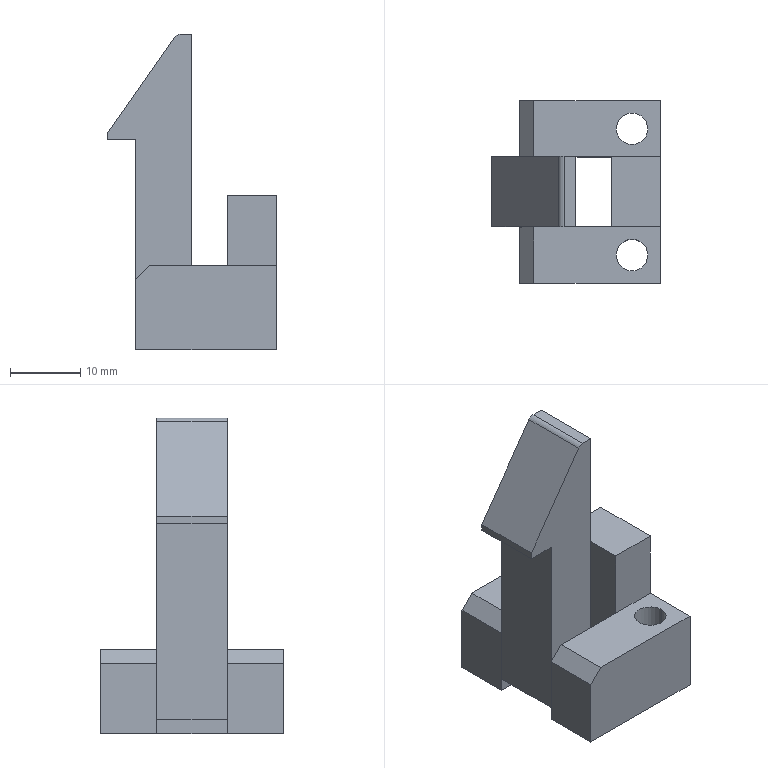Part | SolidWorks | features ICE 4, Chamfer 1, Extrusion 1, Fillet 1 | 2 solids | 30 faces | box 24 x 26 x 45 mm | volume 8320 mm3 | plane 25 | cylinder 5 | commonest cylinder face diameters 4.5 x4 2 x1
STEP:
#1=CARTESIAN_POINT('',(8.25,-9.,0.));
#2=VERTEX_POINT('',#1);
#3=CARTESIAN_POINT('',(3.75,-9.,0.));
#4=VERTEX_POINT('',#3);
#5=CARTESIAN_POINT('',(6.,-9.,0.));
#6=DIRECTION('',(0.,0.,-1.));
#7=DIRECTION('',(1.,0.,0.));
#8=AXIS2_PLACEMENT_3D('',#5,#6,#7);
#9=CIRCLE('',#8,2.25);
#10=EDGE_CURVE('',#2,#4,#9,.T.);
#11=ORIENTED_EDGE('',*,*,#10,.T.);
#12=CARTESIAN_POINT('',(3.75,-9.,12.));
#13=VERTEX_POINT('',#12);
#14=CARTESIAN_POINT('',(3.75,-9.,-0.001));
#15=DIRECTION('',(0.,0.,1.));
#16=VECTOR('',#15,1000.);
#17=LINE('',#14,#16);
#18=EDGE_CURVE('',#4,#13,#17,.T.);
#19=ORIENTED_EDGE('',*,*,#18,.T.);
#20=CARTESIAN_POINT('',(8.25,-9.,12.));
#21=VERTEX_POINT('',#20);
#22=CARTESIAN_POINT('',(6.,-9.,12.));
#23=DIRECTION('',(0.,0.,1.));
#24=DIRECTION('',(1.,0.,0.));
#25=AXIS2_PLACEMENT_3D('',#22,#23,#24);
#26=CIRCLE('',#25,2.25);
#27=EDGE_CURVE('',#13,#21,#26,.T.);
#28=ORIENTED_EDGE('',*,*,#27,.T.);
#29=CARTESIAN_POINT('',(8.25,-9.,-0.001));
#30=DIRECTION('',(0.,0.,1.));
#31=VECTOR('',#30,1000.);
#32=LINE('',#29,#31);
#33=EDGE_CURVE('',#2,#21,#32,.T.);
#34=ORIENTED_EDGE('',*,*,#33,.F.);
#35=EDGE_LOOP('',(#11,#19,#28,#34));
#36=FACE_OUTER_BOUND('',#35,.T.);
#37=CARTESIAN_POINT('',(6.,-9.,-0.001));
#38=DIRECTION('',(0.,0.,1.));
#39=DIRECTION('',(1.,0.,0.));
#40=AXIS2_PLACEMENT_3D('',#37,#38,#39);
#41=CYLINDRICAL_SURFACE('',#40,2.25);
#42=ADVANCED_FACE('',(#36),#41,.F.);
#43=CARTESIAN_POINT('',(8.25,9.,0.));
#44=VERTEX_POINT('',#43);
#45=CARTESIAN_POINT('',(3.75,9.,0.));
#46=VERTEX_POINT('',#45);
#47=CARTESIAN_POINT('',(6.,9.,0.));
#48=DIRECTION('',(0.,0.,-1.));
#49=DIRECTION('',(1.,0.,0.));
#50=AXIS2_PLACEMENT_3D('',#47,#48,#49);
#51=CIRCLE('',#50,2.25);
#52=EDGE_CURVE('',#44,#46,#51,.T.);
#53=ORIENTED_EDGE('',*,*,#52,.T.);
#54=CARTESIAN_POINT('',(3.75,9.,12.));
#55=VERTEX_POINT('',#54);
#56=CARTESIAN_POINT('',(3.75,9.,-0.001));
#57=DIRECTION('',(0.,0.,1.));
#58=VECTOR('',#57,1000.);
#59=LINE('',#56,#58);
#60=EDGE_CURVE('',#46,#55,#59,.T.);
#61=ORIENTED_EDGE('',*,*,#60,.T.);
#62=CARTESIAN_POINT('',(8.25,9.,12.));
#63=VERTEX_POINT('',#62);
#64=CARTESIAN_POINT('',(6.,9.,12.));
#65=DIRECTION('',(0.,0.,1.));
#66=DIRECTION('',(1.,0.,0.));
#67=AXIS2_PLACEMENT_3D('',#64,#65,#66);
#68=CIRCLE('',#67,2.25);
#69=EDGE_CURVE('',#55,#63,#68,.T.);
#70=ORIENTED_EDGE('',*,*,#69,.T.);
#71=CARTESIAN_POINT('',(8.25,9.,-0.001));
#72=DIRECTION('',(0.,0.,1.));
#73=VECTOR('',#72,1000.);
#74=LINE('',#71,#73);
#75=EDGE_CURVE('',#44,#63,#74,.T.);
#76=ORIENTED_EDGE('',*,*,#75,.F.);
#77=EDGE_LOOP('',(#53,#61,#70,#76));
#78=FACE_OUTER_BOUND('',#77,.T.);
#79=CARTESIAN_POINT('',(6.,9.,-0.001));
#80=DIRECTION('',(0.,0.,1.));
#81=DIRECTION('',(1.,0.,0.));
#82=AXIS2_PLACEMENT_3D('',#79,#80,#81);
#83=CYLINDRICAL_SURFACE('',#82,2.25);
#84=ADVANCED_FACE('',(#78),#83,.F.);
#85=CARTESIAN_POINT('',(-10.,-13.,10.));
#86=VERTEX_POINT('',#85);
#87=CARTESIAN_POINT('',(-10.,-13.,0.));
#88=VERTEX_POINT('',#87);
#89=CARTESIAN_POINT('',(-10.,-13.,12.));
#90=DIRECTION('',(0.,0.,-1.));
#91=VECTOR('',#90,1000.);
#92=LINE('',#89,#91);
#93=EDGE_CURVE('',#86,#88,#92,.T.);
#94=ORIENTED_EDGE('',*,*,#93,.F.);
#95=CARTESIAN_POINT('',(-10.,-5.,10.));
#96=VERTEX_POINT('',#95);
#97=CARTESIAN_POINT('',(-10.,-5.,10.));
#98=DIRECTION('',(0.,1.,0.));
#99=VECTOR('',#98,1000.);
#100=LINE('',#97,#99);
#101=EDGE_CURVE('',#86,#96,#100,.T.);
#102=ORIENTED_EDGE('',*,*,#101,.T.);
#103=CARTESIAN_POINT('',(-10.,-5.,0.));
#104=VERTEX_POINT('',#103);
#105=CARTESIAN_POINT('',(-10.,-5.,-0.001));
#106=DIRECTION('',(0.,0.,1.));
#107=VECTOR('',#106,1000.);
#108=LINE('',#105,#107);
#109=EDGE_CURVE('',#104,#96,#108,.T.);
#110=ORIENTED_EDGE('',*,*,#109,.F.);
#111=CARTESIAN_POINT('',(-10.,-13.,0.));
#112=DIRECTION('',(0.,-1.,0.));
#113=VECTOR('',#112,1000.);
#114=LINE('',#111,#113);
#115=EDGE_CURVE('',#104,#88,#114,.T.);
#116=ORIENTED_EDGE('',*,*,#115,.T.);
#117=EDGE_LOOP('',(#94,#102,#110,#116));
#118=FACE_OUTER_BOUND('',#117,.T.);
#119=CARTESIAN_POINT('',(-10.,-13.,12.));
#120=DIRECTION('',(1.,0.,0.));
#121=DIRECTION('',(0.,0.,-1.));
#122=AXIS2_PLACEMENT_3D('',#119,#120,#121);
#123=PLANE('',#122);
#124=ADVANCED_FACE('',(#118),#123,.F.);
#125=CARTESIAN_POINT('',(-8.,-5.,12.));
#126=VERTEX_POINT('',#125);
#127=CARTESIAN_POINT('',(3.,-5.,12.));
#128=VERTEX_POINT('',#127);
#129=CARTESIAN_POINT('',(3.,-5.,12.));
#130=DIRECTION('',(1.,0.,0.));
#131=VECTOR('',#130,1000.);
#132=LINE('',#129,#131);
#133=EDGE_CURVE('',#126,#128,#132,.T.);
#134=ORIENTED_EDGE('',*,*,#133,.F.);
#135=CARTESIAN_POINT('',(-8.,-13.,12.));
#136=VERTEX_POINT('',#135);
#137=CARTESIAN_POINT('',(-8.,-13.,12.));
#138=DIRECTION('',(0.,-1.,0.));
#139=VECTOR('',#138,1000.);
#140=LINE('',#137,#139);
#141=EDGE_CURVE('',#126,#136,#140,.T.);
#142=ORIENTED_EDGE('',*,*,#141,.T.);
#143=CARTESIAN_POINT('',(10.,-13.,12.));
#144=VERTEX_POINT('',#143);
#145=CARTESIAN_POINT('',(10.,-13.,12.));
#146=DIRECTION('',(1.,0.,0.));
#147=VECTOR('',#146,1000.);
#148=LINE('',#145,#147);
#149=EDGE_CURVE('',#136,#144,#148,.T.);
#150=ORIENTED_EDGE('',*,*,#149,.T.);
#151=CARTESIAN_POINT('',(10.,-5.,12.));
#152=VERTEX_POINT('',#151);
#153=CARTESIAN_POINT('',(10.,-13.,12.));
#154=DIRECTION('',(0.,1.,0.));
#155=VECTOR('',#154,1000.);
#156=LINE('',#153,#155);
#157=EDGE_CURVE('',#144,#152,#156,.T.);
#158=ORIENTED_EDGE('',*,*,#157,.T.);
#159=CARTESIAN_POINT('',(10.,-5.,12.));
#160=DIRECTION('',(1.,0.,0.));
#161=VECTOR('',#160,1000.);
#162=LINE('',#159,#161);
#163=EDGE_CURVE('',#128,#152,#162,.T.);
#164=ORIENTED_EDGE('',*,*,#163,.F.);
#165=EDGE_LOOP('',(#134,#142,#150,#158,#164));
#166=FACE_OUTER_BOUND('',#165,.T.);
#167=CARTESIAN_POINT('',(6.,-9.,12.));
#168=DIRECTION('',(0.,0.,1.));
#169=DIRECTION('',(1.,0.,0.));
#170=AXIS2_PLACEMENT_3D('',#167,#168,#169);
#171=CIRCLE('',#170,2.25);
#172=EDGE_CURVE('',#21,#13,#171,.T.);
#173=ORIENTED_EDGE('',*,*,#172,.F.);
#174=ORIENTED_EDGE('',*,*,#27,.F.);
#175=EDGE_LOOP('',(#173,#174));
#176=FACE_BOUND('',#175,.T.);
#177=CARTESIAN_POINT('',(0.,0.,12.));
#178=DIRECTION('',(0.,0.,1.));
#179=DIRECTION('',(1.,0.,0.));
#180=AXIS2_PLACEMENT_3D('',#177,#178,#179);
#181=PLANE('',#180);
#182=ADVANCED_FACE('',(#166,#176),#181,.T.);
#183=CARTESIAN_POINT('',(-10.,5.,0.));
#184=VERTEX_POINT('',#183);
#185=CARTESIAN_POINT('',(-10.,5.,10.));
#186=VERTEX_POINT('',#185);
#187=CARTESIAN_POINT('',(-10.,5.,-0.001));
#188=DIRECTION('',(0.,0.,1.));
#189=VECTOR('',#188,1000.);
#190=LINE('',#187,#189);
#191=EDGE_CURVE('',#184,#186,#190,.T.);
#192=ORIENTED_EDGE('',*,*,#191,.T.);
#193=CARTESIAN_POINT('',(-10.,13.,10.));
#194=VERTEX_POINT('',#193);
#195=CARTESIAN_POINT('',(-10.,13.,10.));
#196=DIRECTION('',(0.,1.,0.));
#197=VECTOR('',#196,1000.);
#198=LINE('',#195,#197);
#199=EDGE_CURVE('',#186,#194,#198,.T.);
#200=ORIENTED_EDGE('',*,*,#199,.T.);
#201=CARTESIAN_POINT('',(-10.,13.,0.));
#202=VERTEX_POINT('',#201);
#203=CARTESIAN_POINT('',(-10.,13.,12.));
#204=DIRECTION('',(0.,0.,-1.));
#205=VECTOR('',#204,1000.);
#206=LINE('',#203,#205);
#207=EDGE_CURVE('',#194,#202,#206,.T.);
#208=ORIENTED_EDGE('',*,*,#207,.T.);
#209=CARTESIAN_POINT('',(-10.,-13.,0.));
#210=DIRECTION('',(0.,-1.,0.));
#211=VECTOR('',#210,1000.);
#212=LINE('',#209,#211);
#213=EDGE_CURVE('',#202,#184,#212,.T.);
#214=ORIENTED_EDGE('',*,*,#213,.T.);
#215=EDGE_LOOP('',(#192,#200,#208,#214));
#216=FACE_OUTER_BOUND('',#215,.T.);
#217=CARTESIAN_POINT('',(-10.,-13.,12.));
#218=DIRECTION('',(1.,0.,0.));
#219=DIRECTION('',(0.,0.,-1.));
#220=AXIS2_PLACEMENT_3D('',#217,#218,#219);
#221=PLANE('',#220);
#222=ADVANCED_FACE('',(#216),#221,.F.);
#223=ORIENTED_EDGE('',*,*,#149,.F.);
#224=CARTESIAN_POINT('',(-8.,-13.,12.));
#225=DIRECTION('',(-0.7071,0.,-0.7071));
#226=VECTOR('',#225,1000.);
#227=LINE('',#224,#226);
#228=EDGE_CURVE('',#136,#86,#227,.T.);
#229=ORIENTED_EDGE('',*,*,#228,.T.);
#230=ORIENTED_EDGE('',*,*,#93,.T.);
#231=CARTESIAN_POINT('',(10.,-13.,0.));
#232=VERTEX_POINT('',#231);
#233=CARTESIAN_POINT('',(10.,-13.,0.));
#234=DIRECTION('',(1.,0.,0.));
#235=VECTOR('',#234,1000.);
#236=LINE('',#233,#235);
#237=EDGE_CURVE('',#88,#232,#236,.T.);
#238=ORIENTED_EDGE('',*,*,#237,.T.);
#239=CARTESIAN_POINT('',(10.,-13.,12.));
#240=DIRECTION('',(0.,0.,-1.));
#241=VECTOR('',#240,1000.);
#242=LINE('',#239,#241);
#243=EDGE_CURVE('',#144,#232,#242,.T.);
#244=ORIENTED_EDGE('',*,*,#243,.F.);
#245=EDGE_LOOP('',(#223,#229,#230,#238,#244));
#246=FACE_OUTER_BOUND('',#245,.T.);
#247=CARTESIAN_POINT('',(10.,-13.,12.));
#248=DIRECTION('',(0.,1.,0.));
#249=DIRECTION('',(-1.,0.,0.));
#250=AXIS2_PLACEMENT_3D('',#247,#248,#249);
#251=PLANE('',#250);
#252=ADVANCED_FACE('',(#246),#251,.F.);
#253=CARTESIAN_POINT('',(10.,13.,0.));
#254=VERTEX_POINT('',#253);
#255=CARTESIAN_POINT('',(10.,-13.,0.));
#256=DIRECTION('',(0.,1.,0.));
#257=VECTOR('',#256,1000.);
#258=LINE('',#255,#257);
#259=EDGE_CURVE('',#232,#254,#258,.T.);
#260=ORIENTED_EDGE('',*,*,#259,.T.);
#261=CARTESIAN_POINT('',(10.,13.,12.));
#262=VERTEX_POINT('',#261);
#263=CARTESIAN_POINT('',(10.,13.,12.));
#264=DIRECTION('',(0.,0.,-1.));
#265=VECTOR('',#264,1000.);
#266=LINE('',#263,#265);
#267=EDGE_CURVE('',#262,#254,#266,.T.);
#268=ORIENTED_EDGE('',*,*,#267,.F.);
#269=CARTESIAN_POINT('',(10.,5.,12.));
#270=VERTEX_POINT('',#269);
#271=CARTESIAN_POINT('',(10.,-13.,12.));
#272=DIRECTION('',(0.,1.,0.));
#273=VECTOR('',#272,1000.);
#274=LINE('',#271,#273);
#275=EDGE_CURVE('',#270,#262,#274,.T.);
#276=ORIENTED_EDGE('',*,*,#275,.F.);
#277=CARTESIAN_POINT('',(10.,5.,22.));
#278=VERTEX_POINT('',#277);
#279=CARTESIAN_POINT('',(10.,5.,22.));
#280=DIRECTION('',(0.,0.,-1.));
#281=VECTOR('',#280,1000.);
#282=LINE('',#279,#281);
#283=EDGE_CURVE('',#278,#270,#282,.T.);
#284=ORIENTED_EDGE('',*,*,#283,.F.);
#285=CARTESIAN_POINT('',(10.,-5.,22.));
#286=VERTEX_POINT('',#285);
#287=CARTESIAN_POINT('',(10.,5.,22.));
#288=DIRECTION('',(0.,1.,0.));
#289=VECTOR('',#288,1000.);
#290=LINE('',#287,#289);
#291=EDGE_CURVE('',#286,#278,#290,.T.);
#292=ORIENTED_EDGE('',*,*,#291,.F.);
#293=CARTESIAN_POINT('',(10.,-5.,22.));
#294=DIRECTION('',(0.,0.,-1.));
#295=VECTOR('',#294,1000.);
#296=LINE('',#293,#295);
#297=EDGE_CURVE('',#286,#152,#296,.T.);
#298=ORIENTED_EDGE('',*,*,#297,.T.);
#299=ORIENTED_EDGE('',*,*,#157,.F.);
#300=ORIENTED_EDGE('',*,*,#243,.T.);
#301=EDGE_LOOP('',(#260,#268,#276,#284,#292,#298,#299,#300));
#302=FACE_OUTER_BOUND('',#301,.T.);
#303=CARTESIAN_POINT('',(10.,-13.,12.));
#304=DIRECTION('',(-1.,0.,0.));
#305=DIRECTION('',(0.,0.,1.));
#306=AXIS2_PLACEMENT_3D('',#303,#304,#305);
#307=PLANE('',#306);
#308=ADVANCED_FACE('',(#302),#307,.F.);
#309=ORIENTED_EDGE('',*,*,#207,.F.);
#310=CARTESIAN_POINT('',(-8.,13.,12.));
#311=VERTEX_POINT('',#310);
#312=CARTESIAN_POINT('',(-8.,13.,12.));
#313=DIRECTION('',(0.7071,0.,0.7071));
#314=VECTOR('',#313,1000.);
#315=LINE('',#312,#314);
#316=EDGE_CURVE('',#194,#311,#315,.T.);
#317=ORIENTED_EDGE('',*,*,#316,.T.);
#318=CARTESIAN_POINT('',(10.,13.,12.));
#319=DIRECTION('',(-1.,0.,0.));
#320=VECTOR('',#319,1000.);
#321=LINE('',#318,#320);
#322=EDGE_CURVE('',#262,#311,#321,.T.);
#323=ORIENTED_EDGE('',*,*,#322,.F.);
#324=ORIENTED_EDGE('',*,*,#267,.T.);
#325=CARTESIAN_POINT('',(10.,13.,0.));
#326=DIRECTION('',(-1.,0.,0.));
#327=VECTOR('',#326,1000.);
#328=LINE('',#325,#327);
#329=EDGE_CURVE('',#254,#202,#328,.T.);
#330=ORIENTED_EDGE('',*,*,#329,.T.);
#331=EDGE_LOOP('',(#309,#317,#323,#324,#330));
#332=FACE_OUTER_BOUND('',#331,.T.);
#333=CARTESIAN_POINT('',(10.,13.,12.));
#334=DIRECTION('',(0.,-1.,0.));
#335=DIRECTION('',(1.,0.,0.));
#336=AXIS2_PLACEMENT_3D('',#333,#334,#335);
#337=PLANE('',#336);
#338=ADVANCED_FACE('',(#332),#337,.F.);
#339=ORIENTED_EDGE('',*,*,#322,.T.);
#340=CARTESIAN_POINT('',(-8.,5.,12.));
#341=VERTEX_POINT('',#340);
#342=CARTESIAN_POINT('',(-8.,5.,12.));
#343=DIRECTION('',(0.,-1.,0.));
#344=VECTOR('',#343,1000.);
#345=LINE('',#342,#344);
#346=EDGE_CURVE('',#311,#341,#345,.T.);
#347=ORIENTED_EDGE('',*,*,#346,.T.);
#348=CARTESIAN_POINT('',(3.,5.,12.));
#349=VERTEX_POINT('',#348);
#350=CARTESIAN_POINT('',(3.,5.,12.));
#351=DIRECTION('',(-1.,0.,0.));
#352=VECTOR('',#351,1000.);
#353=LINE('',#350,#352);
#354=EDGE_CURVE('',#349,#341,#353,.T.);
#355=ORIENTED_EDGE('',*,*,#354,.F.);
#356=CARTESIAN_POINT('',(10.,5.,12.));
#357=DIRECTION('',(-1.,0.,0.));
#358=VECTOR('',#357,1000.);
#359=LINE('',#356,#358);
#360=EDGE_CURVE('',#270,#349,#359,.T.);
#361=ORIENTED_EDGE('',*,*,#360,.F.);
#362=ORIENTED_EDGE('',*,*,#275,.T.);
#363=EDGE_LOOP('',(#339,#347,#355,#361,#362));
#364=FACE_OUTER_BOUND('',#363,.T.);
#365=CARTESIAN_POINT('',(6.,9.,12.));
#366=DIRECTION('',(0.,0.,1.));
#367=DIRECTION('',(1.,0.,0.));
#368=AXIS2_PLACEMENT_3D('',#365,#366,#367);
#369=CIRCLE('',#368,2.25);
#370=EDGE_CURVE('',#63,#55,#369,.T.);
#371=ORIENTED_EDGE('',*,*,#370,.F.);
#372=ORIENTED_EDGE('',*,*,#69,.F.);
#373=EDGE_LOOP('',(#371,#372));
#374=FACE_BOUND('',#373,.T.);
#375=CARTESIAN_POINT('',(0.,0.,12.));
#376=DIRECTION('',(0.,0.,1.));
#377=DIRECTION('',(1.,0.,0.));
#378=AXIS2_PLACEMENT_3D('',#375,#376,#377);
#379=PLANE('',#378);
#380=ADVANCED_FACE('',(#364,#374),#379,.T.);
#381=ORIENTED_EDGE('',*,*,#10,.F.);
#382=CARTESIAN_POINT('',(6.,-9.,0.));
#383=DIRECTION('',(0.,0.,-1.));
#384=DIRECTION('',(1.,0.,0.));
#385=AXIS2_PLACEMENT_3D('',#382,#383,#384);
#386=CIRCLE('',#385,2.25);
#387=EDGE_CURVE('',#4,#2,#386,.T.);
#388=ORIENTED_EDGE('',*,*,#387,.F.);
#389=EDGE_LOOP('',(#381,#388));
#390=FACE_BOUND('',#389,.T.);
#391=ORIENTED_EDGE('',*,*,#52,.F.);
#392=CARTESIAN_POINT('',(6.,9.,0.));
#393=DIRECTION('',(0.,0.,-1.));
#394=DIRECTION('',(1.,0.,0.));
#395=AXIS2_PLACEMENT_3D('',#392,#393,#394);
#396=CIRCLE('',#395,2.25);
#397=EDGE_CURVE('',#46,#44,#396,.T.);
#398=ORIENTED_EDGE('',*,*,#397,.F.);
#399=EDGE_LOOP('',(#391,#398));
#400=FACE_BOUND('',#399,.T.);
#401=ORIENTED_EDGE('',*,*,#115,.F.);
#402=CARTESIAN_POINT('',(3.,-5.,0.));
#403=VERTEX_POINT('',#402);
#404=CARTESIAN_POINT('',(3.,-5.,0.));
#405=DIRECTION('',(-1.,0.,0.));
#406=VECTOR('',#405,1000.);
#407=LINE('',#404,#406);
#408=EDGE_CURVE('',#403,#104,#407,.T.);
#409=ORIENTED_EDGE('',*,*,#408,.F.);
#410=CARTESIAN_POINT('',(3.,5.,0.));
#411=VERTEX_POINT('',#410);
#412=CARTESIAN_POINT('',(3.,5.,0.));
#413=DIRECTION('',(0.,-1.,0.));
#414=VECTOR('',#413,1000.);
#415=LINE('',#412,#414);
#416=EDGE_CURVE('',#411,#403,#415,.T.);
#417=ORIENTED_EDGE('',*,*,#416,.F.);
#418=CARTESIAN_POINT('',(3.,5.,0.));
#419=DIRECTION('',(1.,0.,0.));
#420=VECTOR('',#419,1000.);
#421=LINE('',#418,#420);
#422=EDGE_CURVE('',#184,#411,#421,.T.);
#423=ORIENTED_EDGE('',*,*,#422,.F.);
#424=ORIENTED_EDGE('',*,*,#213,.F.);
#425=ORIENTED_EDGE('',*,*,#329,.F.);
#426=ORIENTED_EDGE('',*,*,#259,.F.);
#427=ORIENTED_EDGE('',*,*,#237,.F.);
#428=EDGE_LOOP('',(#401,#409,#417,#423,#424,#425,#426,#427));
#429=FACE_OUTER_BOUND('',#428,.T.);
#430=CARTESIAN_POINT('',(0.,0.,0.));
#431=DIRECTION('',(0.,0.,1.));
#432=DIRECTION('',(1.,0.,0.));
#433=AXIS2_PLACEMENT_3D('',#430,#431,#432);
#434=PLANE('',#433);
#435=ADVANCED_FACE('',(#390,#400,#429),#434,.F.);
#436=ORIENTED_EDGE('',*,*,#60,.F.);
#437=ORIENTED_EDGE('',*,*,#397,.T.);
#438=ORIENTED_EDGE('',*,*,#75,.T.);
#439=ORIENTED_EDGE('',*,*,#370,.T.);
#440=EDGE_LOOP('',(#436,#437,#438,#439));
#441=FACE_OUTER_BOUND('',#440,.T.);
#442=CARTESIAN_POINT('',(6.,9.,-0.001));
#443=DIRECTION('',(0.,0.,1.));
#444=DIRECTION('',(1.,0.,0.));
#445=AXIS2_PLACEMENT_3D('',#442,#443,#444);
#446=CYLINDRICAL_SURFACE('',#445,2.25);
#447=ADVANCED_FACE('',(#441),#446,.F.);
#448=ORIENTED_EDGE('',*,*,#18,.F.);
#449=ORIENTED_EDGE('',*,*,#387,.T.);
#450=ORIENTED_EDGE('',*,*,#33,.T.);
#451=ORIENTED_EDGE('',*,*,#172,.T.);
#452=EDGE_LOOP('',(#448,#449,#450,#451));
#453=FACE_OUTER_BOUND('',#452,.T.);
#454=CARTESIAN_POINT('',(6.,-9.,-0.001));
#455=DIRECTION('',(0.,0.,1.));
#456=DIRECTION('',(1.,0.,0.));
#457=AXIS2_PLACEMENT_3D('',#454,#455,#456);
#458=CYLINDRICAL_SURFACE('',#457,2.25);
#459=ADVANCED_FACE('',(#453),#458,.F.);
#460=ORIENTED_EDGE('',*,*,#360,.T.);
#461=CARTESIAN_POINT('',(3.,5.,22.));
#462=VERTEX_POINT('',#461);
#463=CARTESIAN_POINT('',(3.,5.,22.));
#464=DIRECTION('',(0.,0.,-1.));
#465=VECTOR('',#464,1000.);
#466=LINE('',#463,#465);
#467=EDGE_CURVE('',#462,#349,#466,.T.);
#468=ORIENTED_EDGE('',*,*,#467,.F.);
#469=CARTESIAN_POINT('',(10.,5.,22.));
#470=DIRECTION('',(-1.,0.,0.));
#471=VECTOR('',#470,1000.);
#472=LINE('',#469,#471);
#473=EDGE_CURVE('',#278,#462,#472,.T.);
#474=ORIENTED_EDGE('',*,*,#473,.F.);
#475=ORIENTED_EDGE('',*,*,#283,.T.);
#476=EDGE_LOOP('',(#460,#468,#474,#475));
#477=FACE_OUTER_BOUND('',#476,.T.);
#478=CARTESIAN_POINT('',(10.,5.,22.));
#479=DIRECTION('',(0.,-1.,0.));
#480=DIRECTION('',(1.,0.,0.));
#481=AXIS2_PLACEMENT_3D('',#478,#479,#480);
#482=PLANE('',#481);
#483=ADVANCED_FACE('',(#477),#482,.F.);
#484=ORIENTED_EDGE('',*,*,#467,.T.);
#485=CARTESIAN_POINT('',(3.,5.,-0.001));
#486=DIRECTION('',(0.,0.,1.));
#487=VECTOR('',#486,1000.);
#488=LINE('',#485,#487);
#489=EDGE_CURVE('',#411,#349,#488,.T.);
#490=ORIENTED_EDGE('',*,*,#489,.F.);
#491=ORIENTED_EDGE('',*,*,#416,.T.);
#492=CARTESIAN_POINT('',(3.,-5.,-0.001));
#493=DIRECTION('',(0.,0.,1.));
#494=VECTOR('',#493,1000.);
#495=LINE('',#492,#494);
#496=EDGE_CURVE('',#403,#128,#495,.T.);
#497=ORIENTED_EDGE('',*,*,#496,.T.);
#498=CARTESIAN_POINT('',(3.,-5.,22.));
#499=VERTEX_POINT('',#498);
#500=CARTESIAN_POINT('',(3.,-5.,22.));
#501=DIRECTION('',(0.,0.,-1.));
#502=VECTOR('',#501,1000.);
#503=LINE('',#500,#502);
#504=EDGE_CURVE('',#499,#128,#503,.T.);
#505=ORIENTED_EDGE('',*,*,#504,.F.);
#506=CARTESIAN_POINT('',(3.,5.,22.));
#507=DIRECTION('',(0.,-1.,0.));
#508=VECTOR('',#507,1000.);
#509=LINE('',#506,#508);
#510=EDGE_CURVE('',#462,#499,#509,.T.);
#511=ORIENTED_EDGE('',*,*,#510,.F.);
#512=EDGE_LOOP('',(#484,#490,#491,#497,#505,#511));
#513=FACE_OUTER_BOUND('',#512,.T.);
#514=CARTESIAN_POINT('',(3.,5.,22.));
#515=DIRECTION('',(1.,0.,0.));
#516=DIRECTION('',(0.,1.,0.));
#517=AXIS2_PLACEMENT_3D('',#514,#515,#516);
#518=PLANE('',#517);
#519=ADVANCED_FACE('',(#513),#518,.F.);
#520=ORIENTED_EDGE('',*,*,#163,.T.);
#521=ORIENTED_EDGE('',*,*,#297,.F.);
#522=CARTESIAN_POINT('',(10.,-5.,22.));
#523=DIRECTION('',(1.,0.,0.));
#524=VECTOR('',#523,1000.);
#525=LINE('',#522,#524);
#526=EDGE_CURVE('',#499,#286,#525,.T.);
#527=ORIENTED_EDGE('',*,*,#526,.F.);
#528=ORIENTED_EDGE('',*,*,#504,.T.);
#529=EDGE_LOOP('',(#520,#521,#527,#528));
#530=FACE_OUTER_BOUND('',#529,.T.);
#531=CARTESIAN_POINT('',(10.,-5.,22.));
#532=DIRECTION('',(0.,1.,0.));
#533=DIRECTION('',(-1.,0.,0.));
#534=AXIS2_PLACEMENT_3D('',#531,#532,#533);
#535=PLANE('',#534);
#536=ADVANCED_FACE('',(#530),#535,.F.);
#537=ORIENTED_EDGE('',*,*,#291,.T.);
#538=ORIENTED_EDGE('',*,*,#473,.T.);
#539=ORIENTED_EDGE('',*,*,#510,.T.);
#540=ORIENTED_EDGE('',*,*,#526,.T.);
#541=EDGE_LOOP('',(#537,#538,#539,#540));
#542=FACE_OUTER_BOUND('',#541,.T.);
#543=CARTESIAN_POINT('',(0.,0.,22.));
#544=DIRECTION('',(0.,0.,-1.));
#545=DIRECTION('',(-1.,0.,0.));
#546=AXIS2_PLACEMENT_3D('',#543,#544,#545);
#547=PLANE('',#546);
#548=ADVANCED_FACE('',(#542),#547,.F.);
#549=ORIENTED_EDGE('',*,*,#109,.T.);
#550=CARTESIAN_POINT('',(-8.,-5.,12.));
#551=DIRECTION('',(0.7071,0.,0.7071));
#552=VECTOR('',#551,1000.);
#553=LINE('',#550,#552);
#554=EDGE_CURVE('',#96,#126,#553,.T.);
#555=ORIENTED_EDGE('',*,*,#554,.T.);
#556=ORIENTED_EDGE('',*,*,#133,.T.);
#557=ORIENTED_EDGE('',*,*,#496,.F.);
#558=ORIENTED_EDGE('',*,*,#408,.T.);
#559=EDGE_LOOP('',(#549,#555,#556,#557,#558));
#560=FACE_OUTER_BOUND('',#559,.T.);
#561=CARTESIAN_POINT('',(3.,-5.,-0.001));
#562=DIRECTION('',(0.,-1.,0.));
#563=DIRECTION('',(1.,0.,0.));
#564=AXIS2_PLACEMENT_3D('',#561,#562,#563);
#565=PLANE('',#564);
#566=ADVANCED_FACE('',(#560),#565,.F.);
#567=ORIENTED_EDGE('',*,*,#354,.T.);
#568=CARTESIAN_POINT('',(-8.,5.,12.));
#569=DIRECTION('',(-0.7071,0.,-0.7071));
#570=VECTOR('',#569,1000.);
#571=LINE('',#568,#570);
#572=EDGE_CURVE('',#341,#186,#571,.T.);
#573=ORIENTED_EDGE('',*,*,#572,.T.);
#574=ORIENTED_EDGE('',*,*,#191,.F.);
#575=ORIENTED_EDGE('',*,*,#422,.T.);
#576=ORIENTED_EDGE('',*,*,#489,.T.);
#577=EDGE_LOOP('',(#567,#573,#574,#575,#576));
#578=FACE_OUTER_BOUND('',#577,.T.);
#579=CARTESIAN_POINT('',(3.,5.,-0.001));
#580=DIRECTION('',(0.,1.,0.));
#581=DIRECTION('',(-1.,0.,0.));
#582=AXIS2_PLACEMENT_3D('',#579,#580,#581);
#583=PLANE('',#582);
#584=ADVANCED_FACE('',(#578),#583,.F.);
#585=ORIENTED_EDGE('',*,*,#554,.F.);
#586=ORIENTED_EDGE('',*,*,#101,.F.);
#587=ORIENTED_EDGE('',*,*,#228,.F.);
#588=ORIENTED_EDGE('',*,*,#141,.F.);
#589=EDGE_LOOP('',(#585,#586,#587,#588));
#590=FACE_OUTER_BOUND('',#589,.T.);
#591=CARTESIAN_POINT('',(-8.,0.,12.));
#592=DIRECTION('',(-0.7071,0.,0.7071));
#593=DIRECTION('',(0.,1.,0.));
#594=AXIS2_PLACEMENT_3D('',#591,#592,#593);
#595=PLANE('',#594);
#596=ADVANCED_FACE('',(#590),#595,.T.);
#597=ORIENTED_EDGE('',*,*,#316,.F.);
#598=ORIENTED_EDGE('',*,*,#199,.F.);
#599=ORIENTED_EDGE('',*,*,#572,.F.);
#600=ORIENTED_EDGE('',*,*,#346,.F.);
#601=EDGE_LOOP('',(#597,#598,#599,#600));
#602=FACE_OUTER_BOUND('',#601,.T.);
#603=CARTESIAN_POINT('',(-8.,0.,12.));
#604=DIRECTION('',(-0.7071,0.,0.7071));
#605=DIRECTION('',(0.,1.,0.));
#606=AXIS2_PLACEMENT_3D('',#603,#604,#605);
#607=PLANE('',#606);
#608=ADVANCED_FACE('',(#602),#607,.T.);
#609=CLOSED_SHELL('',(#42,#84,#124,#182,#222,#252,#308,#338,#380,#435,#447,#459,#483,#519,#536,#548,#566,#584,#596,#608));
#610=MANIFOLD_SOLID_BREP('',#609);
#611=CARTESIAN_POINT('',(-10.,-5.,2.));
#612=VERTEX_POINT('',#611);
#613=CARTESIAN_POINT('',(-10.,5.,2.));
#614=VERTEX_POINT('',#613);
#615=CARTESIAN_POINT('',(-10.,-5.,2.));
#616=DIRECTION('',(0.,1.,0.));
#617=VECTOR('',#616,1000.);
#618=LINE('',#615,#617);
#619=EDGE_CURVE('',#612,#614,#618,.T.);
#620=ORIENTED_EDGE('',*,*,#619,.T.);
#621=CARTESIAN_POINT('',(-2.,5.,2.));
#622=VERTEX_POINT('',#621);
#623=CARTESIAN_POINT('',(-2.,5.,2.));
#624=DIRECTION('',(-1.,0.,0.));
#625=VECTOR('',#624,1000.);
#626=LINE('',#623,#625);
#627=EDGE_CURVE('',#622,#614,#626,.T.);
#628=ORIENTED_EDGE('',*,*,#627,.F.);
#629=CARTESIAN_POINT('',(-2.,-5.,2.));
#630=VERTEX_POINT('',#629);
#631=CARTESIAN_POINT('',(-2.,-5.,2.));
#632=DIRECTION('',(0.,1.,0.));
#633=VECTOR('',#632,1000.);
#634=LINE('',#631,#633);
#635=EDGE_CURVE('',#630,#622,#634,.T.);
#636=ORIENTED_EDGE('',*,*,#635,.F.);
#637=CARTESIAN_POINT('',(-2.,-5.,2.));
#638=DIRECTION('',(-1.,0.,0.));
#639=VECTOR('',#638,1000.);
#640=LINE('',#637,#639);
#641=EDGE_CURVE('',#630,#612,#640,.T.);
#642=ORIENTED_EDGE('',*,*,#641,.T.);
#643=EDGE_LOOP('',(#620,#628,#636,#642));
#644=FACE_OUTER_BOUND('',#643,.T.);
#645=CARTESIAN_POINT('',(-2.,-5.,2.));
#646=DIRECTION('',(0.,0.,-1.));
#647=DIRECTION('',(-1.,0.,0.));
#648=AXIS2_PLACEMENT_3D('',#645,#646,#647);
#649=PLANE('',#648);
#650=ADVANCED_FACE('',(#644),#649,.T.);
#651=ORIENTED_EDGE('',*,*,#635,.T.);
#652=CARTESIAN_POINT('',(-2.,5.,45.));
#653=VERTEX_POINT('',#652);
#654=CARTESIAN_POINT('',(-2.,5.,45.));
#655=DIRECTION('',(0.,0.,-1.));
#656=VECTOR('',#655,1000.);
#657=LINE('',#654,#656);
#658=EDGE_CURVE('',#653,#622,#657,.T.);
#659=ORIENTED_EDGE('',*,*,#658,.F.);
#660=CARTESIAN_POINT('',(-2.,-5.,45.));
#661=VERTEX_POINT('',#660);
#662=CARTESIAN_POINT('',(-2.,-5.,45.));
#663=DIRECTION('',(0.,1.,0.));
#664=VECTOR('',#663,1000.);
#665=LINE('',#662,#664);
#666=EDGE_CURVE('',#661,#653,#665,.T.);
#667=ORIENTED_EDGE('',*,*,#666,.F.);
#668=CARTESIAN_POINT('',(-2.,-5.,45.));
#669=DIRECTION('',(0.,0.,-1.));
#670=VECTOR('',#669,1000.);
#671=LINE('',#668,#670);
#672=EDGE_CURVE('',#661,#630,#671,.T.);
#673=ORIENTED_EDGE('',*,*,#672,.T.);
#674=EDGE_LOOP('',(#651,#659,#667,#673));
#675=FACE_OUTER_BOUND('',#674,.T.);
#676=CARTESIAN_POINT('',(-2.,-5.,45.));
#677=DIRECTION('',(1.,0.,0.));
#678=DIRECTION('',(0.,0.,-1.));
#679=AXIS2_PLACEMENT_3D('',#676,#677,#678);
#680=PLANE('',#679);
#681=ADVANCED_FACE('',(#675),#680,.T.);
#682=CARTESIAN_POINT('',(-3.677,5.,45.));
#683=VERTEX_POINT('',#682);
#684=CARTESIAN_POINT('',(-4.197,5.,45.));
#685=DIRECTION('',(1.,0.,0.));
#686=VECTOR('',#685,1000.);
#687=LINE('',#684,#686);
#688=EDGE_CURVE('',#683,#653,#687,.T.);
#689=ORIENTED_EDGE('',*,*,#688,.F.);
#690=CARTESIAN_POINT('',(-3.677,-5.,45.));
#691=VERTEX_POINT('',#690);
#692=CARTESIAN_POINT('',(-3.677,-5.,45.));
#693=DIRECTION('',(0.,-1.,0.));
#694=VECTOR('',#693,1000.);
#695=LINE('',#692,#694);
#696=EDGE_CURVE('',#683,#691,#695,.T.);
#697=ORIENTED_EDGE('',*,*,#696,.T.);
#698=CARTESIAN_POINT('',(-4.197,-5.,45.));
#699=DIRECTION('',(1.,0.,0.));
#700=VECTOR('',#699,1000.);
#701=LINE('',#698,#700);
#702=EDGE_CURVE('',#691,#661,#701,.T.);
#703=ORIENTED_EDGE('',*,*,#702,.T.);
#704=ORIENTED_EDGE('',*,*,#666,.T.);
#705=EDGE_LOOP('',(#689,#697,#703,#704));
#706=FACE_OUTER_BOUND('',#705,.T.);
#707=CARTESIAN_POINT('',(-4.197,-5.,45.));
#708=DIRECTION('',(0.,0.,1.));
#709=DIRECTION('',(1.,0.,0.));
#710=AXIS2_PLACEMENT_3D('',#707,#708,#709);
#711=PLANE('',#710);
#712=ADVANCED_FACE('',(#706),#711,.T.);
#713=CARTESIAN_POINT('',(-14.,-5.,31.));
#714=VERTEX_POINT('',#713);
#715=CARTESIAN_POINT('',(-4.496,-5.,44.574));
#716=VERTEX_POINT('',#715);
#717=CARTESIAN_POINT('',(-14.,-5.,31.));
#718=DIRECTION('',(0.5736,0.,0.8192));
#719=VECTOR('',#718,1000.);
#720=LINE('',#717,#719);
#721=EDGE_CURVE('',#714,#716,#720,.T.);
#722=ORIENTED_EDGE('',*,*,#721,.T.);
#723=CARTESIAN_POINT('',(-4.496,5.,44.574));
#724=VERTEX_POINT('',#723);
#725=CARTESIAN_POINT('',(-4.496,-5.,44.574));
#726=DIRECTION('',(0.,1.,0.));
#727=VECTOR('',#726,1000.);
#728=LINE('',#725,#727);
#729=EDGE_CURVE('',#716,#724,#728,.T.);
#730=ORIENTED_EDGE('',*,*,#729,.T.);
#731=CARTESIAN_POINT('',(-14.,5.,31.));
#732=VERTEX_POINT('',#731);
#733=CARTESIAN_POINT('',(-14.,5.,31.));
#734=DIRECTION('',(0.5736,0.,0.8192));
#735=VECTOR('',#734,1000.);
#736=LINE('',#733,#735);
#737=EDGE_CURVE('',#732,#724,#736,.T.);
#738=ORIENTED_EDGE('',*,*,#737,.F.);
#739=CARTESIAN_POINT('',(-14.,-5.,31.));
#740=DIRECTION('',(0.,1.,0.));
#741=VECTOR('',#740,1000.);
#742=LINE('',#739,#741);
#743=EDGE_CURVE('',#714,#732,#742,.T.);
#744=ORIENTED_EDGE('',*,*,#743,.F.);
#745=EDGE_LOOP('',(#722,#730,#738,#744));
#746=FACE_OUTER_BOUND('',#745,.T.);
#747=CARTESIAN_POINT('',(-14.,-5.,31.));
#748=DIRECTION('',(-0.8192,0.,0.5736));
#749=DIRECTION('',(0.5736,0.,0.8192));
#750=AXIS2_PLACEMENT_3D('',#747,#748,#749);
#751=PLANE('',#750);
#752=ADVANCED_FACE('',(#746),#751,.T.);
#753=ORIENTED_EDGE('',*,*,#743,.T.);
#754=CARTESIAN_POINT('',(-14.,5.,30.));
#755=VERTEX_POINT('',#754);
#756=CARTESIAN_POINT('',(-14.,5.,30.));
#757=DIRECTION('',(0.,0.,1.));
#758=VECTOR('',#757,1000.);
#759=LINE('',#756,#758);
#760=EDGE_CURVE('',#755,#732,#759,.T.);
#761=ORIENTED_EDGE('',*,*,#760,.F.);
#762=CARTESIAN_POINT('',(-14.,-5.,30.));
#763=VERTEX_POINT('',#762);
#764=CARTESIAN_POINT('',(-14.,-5.,30.));
#765=DIRECTION('',(0.,1.,0.));
#766=VECTOR('',#765,1000.);
#767=LINE('',#764,#766);
#768=EDGE_CURVE('',#763,#755,#767,.T.);
#769=ORIENTED_EDGE('',*,*,#768,.F.);
#770=CARTESIAN_POINT('',(-14.,-5.,30.));
#771=DIRECTION('',(0.,0.,1.));
#772=VECTOR('',#771,1000.);
#773=LINE('',#770,#772);
#774=EDGE_CURVE('',#763,#714,#773,.T.);
#775=ORIENTED_EDGE('',*,*,#774,.T.);
#776=EDGE_LOOP('',(#753,#761,#769,#775));
#777=FACE_OUTER_BOUND('',#776,.T.);
#778=CARTESIAN_POINT('',(-14.,-5.,30.));
#779=DIRECTION('',(-1.,0.,0.));
#780=DIRECTION('',(0.,0.,1.));
#781=AXIS2_PLACEMENT_3D('',#778,#779,#780);
#782=PLANE('',#781);
#783=ADVANCED_FACE('',(#777),#782,.T.);
#784=ORIENTED_EDGE('',*,*,#768,.T.);
#785=CARTESIAN_POINT('',(-10.,5.,30.));
#786=VERTEX_POINT('',#785);
#787=CARTESIAN_POINT('',(-10.,5.,30.));
#788=DIRECTION('',(-1.,0.,0.));
#789=VECTOR('',#788,1000.);
#790=LINE('',#787,#789);
#791=EDGE_CURVE('',#786,#755,#790,.T.);
#792=ORIENTED_EDGE('',*,*,#791,.F.);
#793=CARTESIAN_POINT('',(-10.,-5.,30.));
#794=VERTEX_POINT('',#793);
#795=CARTESIAN_POINT('',(-10.,-5.,30.));
#796=DIRECTION('',(0.,1.,0.));
#797=VECTOR('',#796,1000.);
#798=LINE('',#795,#797);
#799=EDGE_CURVE('',#794,#786,#798,.T.);
#800=ORIENTED_EDGE('',*,*,#799,.F.);
#801=CARTESIAN_POINT('',(-10.,-5.,30.));
#802=DIRECTION('',(-1.,0.,0.));
#803=VECTOR('',#802,1000.);
#804=LINE('',#801,#803);
#805=EDGE_CURVE('',#794,#763,#804,.T.);
#806=ORIENTED_EDGE('',*,*,#805,.T.);
#807=EDGE_LOOP('',(#784,#792,#800,#806));
#808=FACE_OUTER_BOUND('',#807,.T.);
#809=CARTESIAN_POINT('',(-10.,-5.,30.));
#810=DIRECTION('',(0.,0.,-1.));
#811=DIRECTION('',(-1.,0.,0.));
#812=AXIS2_PLACEMENT_3D('',#809,#810,#811);
#813=PLANE('',#812);
#814=ADVANCED_FACE('',(#808),#813,.T.);
#815=ORIENTED_EDGE('',*,*,#799,.T.);
#816=CARTESIAN_POINT('',(-10.,5.,2.));
#817=DIRECTION('',(0.,0.,1.));
#818=VECTOR('',#817,1000.);
#819=LINE('',#816,#818);
#820=EDGE_CURVE('',#614,#786,#819,.T.);
#821=ORIENTED_EDGE('',*,*,#820,.F.);
#822=ORIENTED_EDGE('',*,*,#619,.F.);
#823=CARTESIAN_POINT('',(-10.,-5.,2.));
#824=DIRECTION('',(0.,0.,1.));
#825=VECTOR('',#824,1000.);
#826=LINE('',#823,#825);
#827=EDGE_CURVE('',#612,#794,#826,.T.);
#828=ORIENTED_EDGE('',*,*,#827,.T.);
#829=EDGE_LOOP('',(#815,#821,#822,#828));
#830=FACE_OUTER_BOUND('',#829,.T.);
#831=CARTESIAN_POINT('',(-10.,-5.,2.));
#832=DIRECTION('',(-1.,0.,0.));
#833=DIRECTION('',(0.,0.,1.));
#834=AXIS2_PLACEMENT_3D('',#831,#832,#833);
#835=PLANE('',#834);
#836=ADVANCED_FACE('',(#830),#835,.T.);
#837=ORIENTED_EDGE('',*,*,#702,.F.);
#838=CARTESIAN_POINT('',(-3.677,-5.,44.));
#839=DIRECTION('',(0.,-1.,0.));
#840=DIRECTION('',(0.,0.,1.));
#841=AXIS2_PLACEMENT_3D('',#838,#839,#840);
#842=CIRCLE('',#841,1.);
#843=EDGE_CURVE('',#691,#716,#842,.T.);
#844=ORIENTED_EDGE('',*,*,#843,.T.);
#845=ORIENTED_EDGE('',*,*,#721,.F.);
#846=ORIENTED_EDGE('',*,*,#774,.F.);
#847=ORIENTED_EDGE('',*,*,#805,.F.);
#848=ORIENTED_EDGE('',*,*,#827,.F.);
#849=ORIENTED_EDGE('',*,*,#641,.F.);
#850=ORIENTED_EDGE('',*,*,#672,.F.);
#851=EDGE_LOOP('',(#837,#844,#845,#846,#847,#848,#849,#850));
#852=FACE_OUTER_BOUND('',#851,.T.);
#853=CARTESIAN_POINT('',(0.,-5.,0.));
#854=DIRECTION('',(0.,1.,0.));
#855=DIRECTION('',(0.,0.,1.));
#856=AXIS2_PLACEMENT_3D('',#853,#854,#855);
#857=PLANE('',#856);
#858=ADVANCED_FACE('',(#852),#857,.F.);
#859=ORIENTED_EDGE('',*,*,#737,.T.);
#860=CARTESIAN_POINT('',(-3.677,5.,44.));
#861=DIRECTION('',(0.,1.,0.));
#862=DIRECTION('',(0.,0.,1.));
#863=AXIS2_PLACEMENT_3D('',#860,#861,#862);
#864=CIRCLE('',#863,1.);
#865=EDGE_CURVE('',#724,#683,#864,.T.);
#866=ORIENTED_EDGE('',*,*,#865,.T.);
#867=ORIENTED_EDGE('',*,*,#688,.T.);
#868=ORIENTED_EDGE('',*,*,#658,.T.);
#869=ORIENTED_EDGE('',*,*,#627,.T.);
#870=ORIENTED_EDGE('',*,*,#820,.T.);
#871=ORIENTED_EDGE('',*,*,#791,.T.);
#872=ORIENTED_EDGE('',*,*,#760,.T.);
#873=EDGE_LOOP('',(#859,#866,#867,#868,#869,#870,#871,#872));
#874=FACE_OUTER_BOUND('',#873,.T.);
#875=CARTESIAN_POINT('',(0.,5.,0.));
#876=DIRECTION('',(0.,1.,0.));
#877=DIRECTION('',(0.,0.,1.));
#878=AXIS2_PLACEMENT_3D('',#875,#876,#877);
#879=PLANE('',#878);
#880=ADVANCED_FACE('',(#874),#879,.T.);
#881=ORIENTED_EDGE('',*,*,#843,.F.);
#882=ORIENTED_EDGE('',*,*,#696,.F.);
#883=ORIENTED_EDGE('',*,*,#865,.F.);
#884=ORIENTED_EDGE('',*,*,#729,.F.);
#885=EDGE_LOOP('',(#881,#882,#883,#884));
#886=FACE_OUTER_BOUND('',#885,.T.);
#887=CARTESIAN_POINT('',(-3.677,-5.,44.));
#888=DIRECTION('',(0.,1.,0.));
#889=DIRECTION('',(0.,0.,1.));
#890=AXIS2_PLACEMENT_3D('',#887,#888,#889);
#891=CYLINDRICAL_SURFACE('',#890,1.);
#892=ADVANCED_FACE('',(#886),#891,.T.);
#893=CLOSED_SHELL('',(#650,#681,#712,#752,#783,#814,#836,#858,#880,#892));
#894=MANIFOLD_SOLID_BREP('',#893);
#895=CARTESIAN_POINT('',(0.,0.,0.));
#896=DIRECTION('',(0.,0.,1.));
#897=DIRECTION('',(1.,0.,0.));
#898=AXIS2_PLACEMENT_3D('',#895,#896,#897);
#899=(LENGTH_UNIT()NAMED_UNIT(*)SI_UNIT(.MILLI.,.METRE.));
#900=UNCERTAINTY_MEASURE_WITH_UNIT(LENGTH_MEASURE(0.00001),#899,'','');
#901=(NAMED_UNIT(*)PLANE_ANGLE_UNIT()SI_UNIT($,.RADIAN.));
#902=(NAMED_UNIT(*)SI_UNIT($,.STERADIAN.)SOLID_ANGLE_UNIT());
#903=(GEOMETRIC_REPRESENTATION_CONTEXT(3)GLOBAL_UNCERTAINTY_ASSIGNED_CONTEXT((#900))GLOBAL_UNIT_ASSIGNED_CONTEXT((#899,#901,#902))REPRESENTATION_CONTEXT('',''));
#904=ADVANCED_BREP_SHAPE_REPRESENTATION('',(#610,#894,#898),#903);